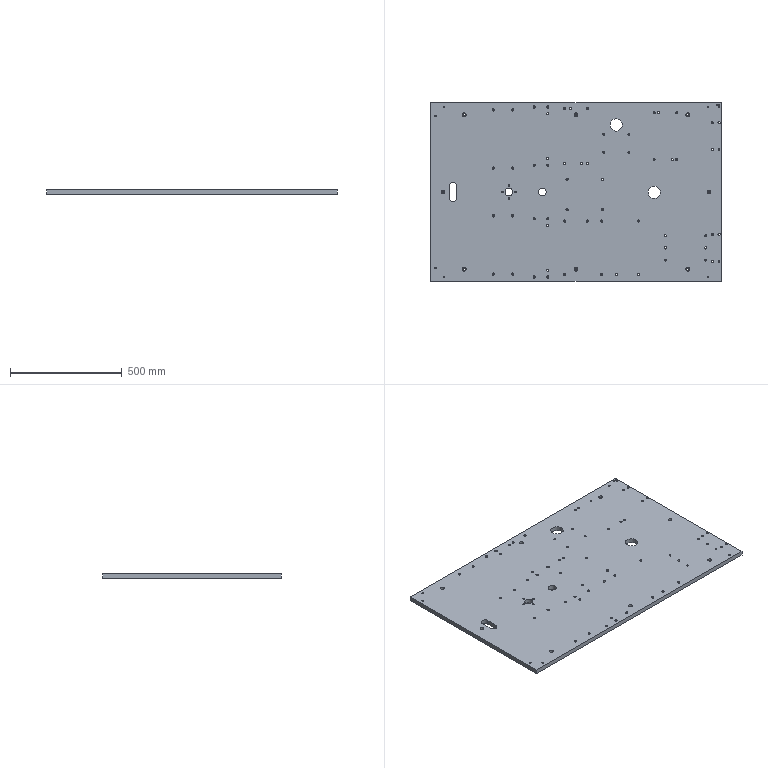Part | STEP file | YBQDJ large plate | 1 solid | 225 faces | box 1300 x 800 x 20 mm | volume 20508106 mm3 | cone 115 | cylinder 94 | plane 16 | commonest cylinder face diameters 8.5 x30 6.8 x26 10 x16 10.7 x8 17 x8 35 x4